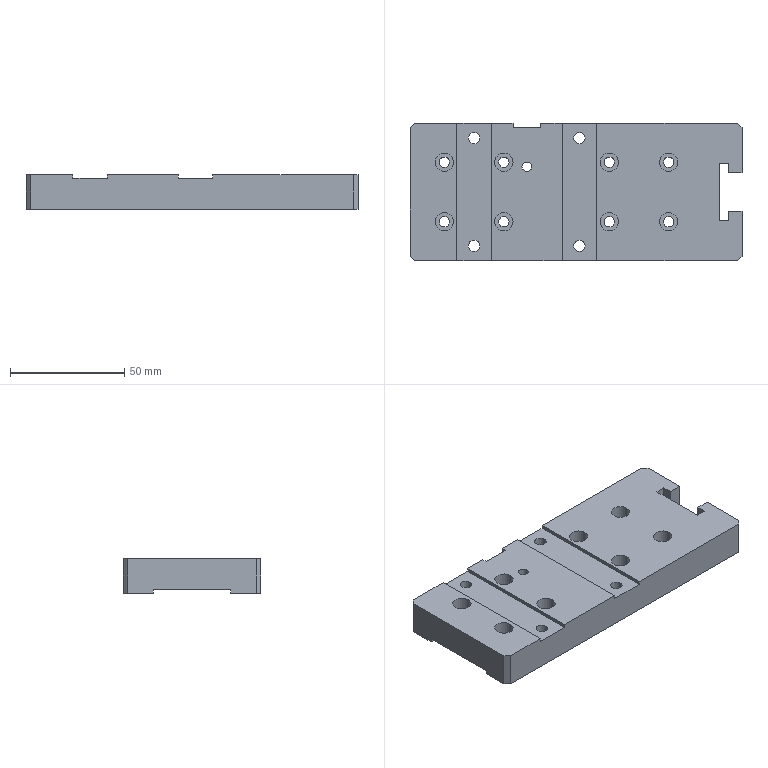Part | STEP file | 11-FG-E01011 | 1 solid | 88 faces | box 145 x 60 x 15 mm | volume 112264 mm3 | cylinder 44 | plane 42 | cone 2 | commonest cylinder face diameters 4.5 x16 8 x16 5 x8 4.2 x4